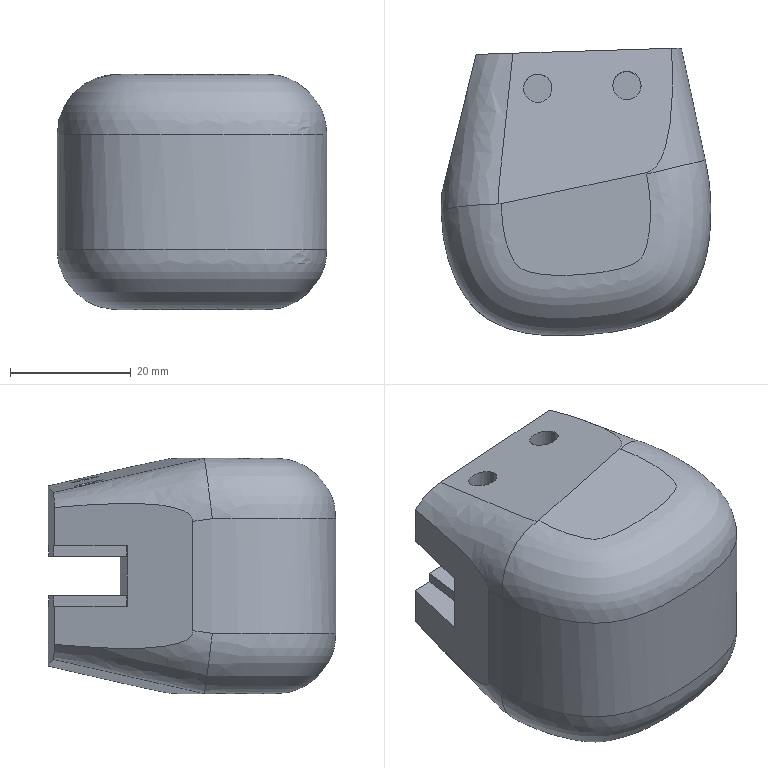Part | SolidWorks | features ICE 6, Extrusion 1, Fillet 1, MirrorPattern 1 | 1 solid | 36 faces | box 44.726 x 47.714 x 39 mm | volume 59211 mm3 | plane 21 | cylinder 10 | spline 5 | commonest cylinder face diameters 4.7 x8 20 x2